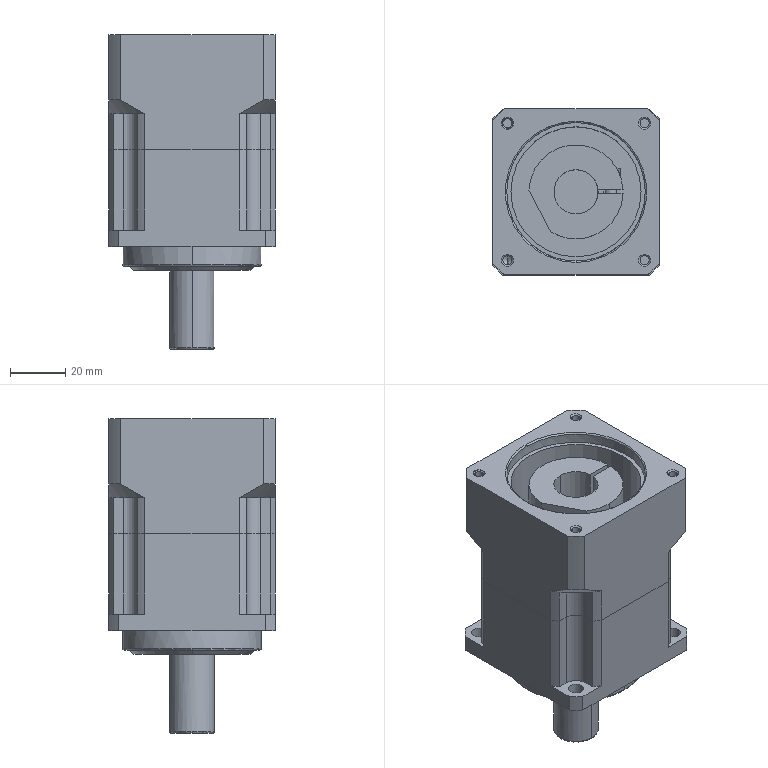Part | NX | 2 solids | 165 faces | box 60 x 60 x 113.5 mm | volume 214912 mm3 | cylinder 76 | plane 61 | cone 20 | torus 8 | commonest cylinder face diameters 69 x16 3.3 x8 5.5 x8 10 x8 4 x4 16 x4